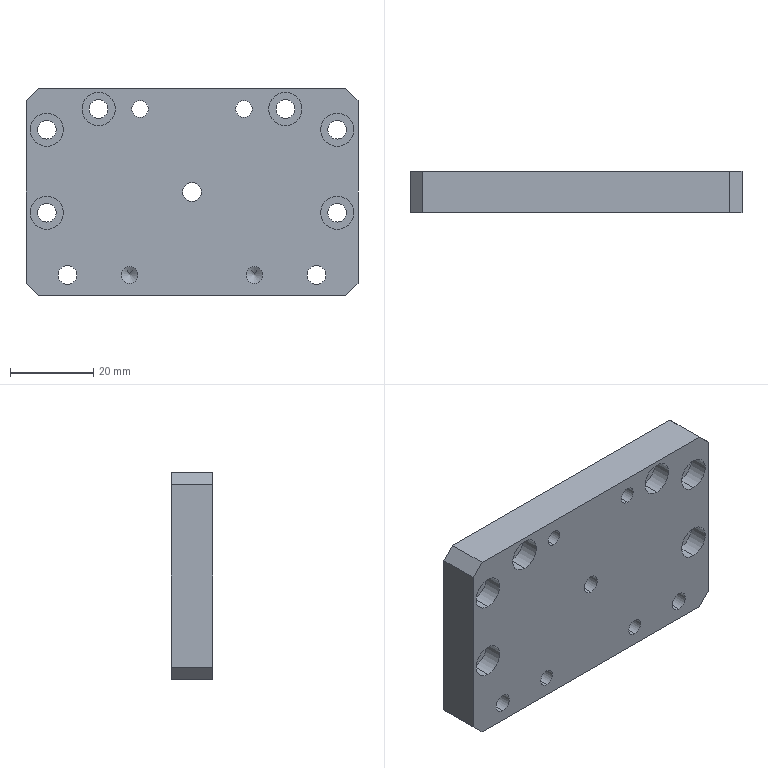Part | STEP file | PN_0020 | 1 solid | 67 faces | box 80 x 10 x 50 mm | volume 36297 mm3 | cylinder 44 | plane 19 | cone 4 | commonest cylinder face diameters 4.5 x18 8 x18 4 x8